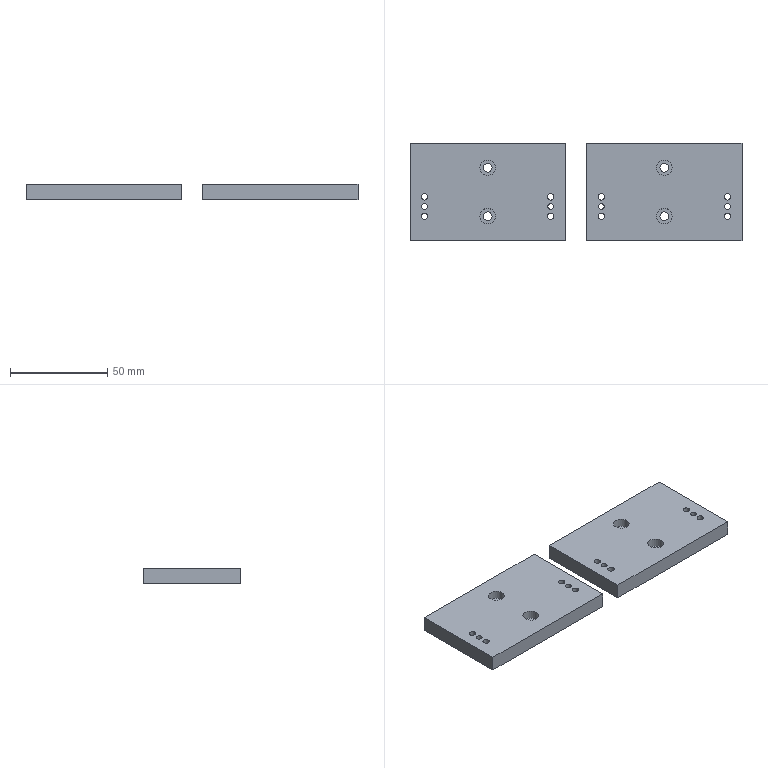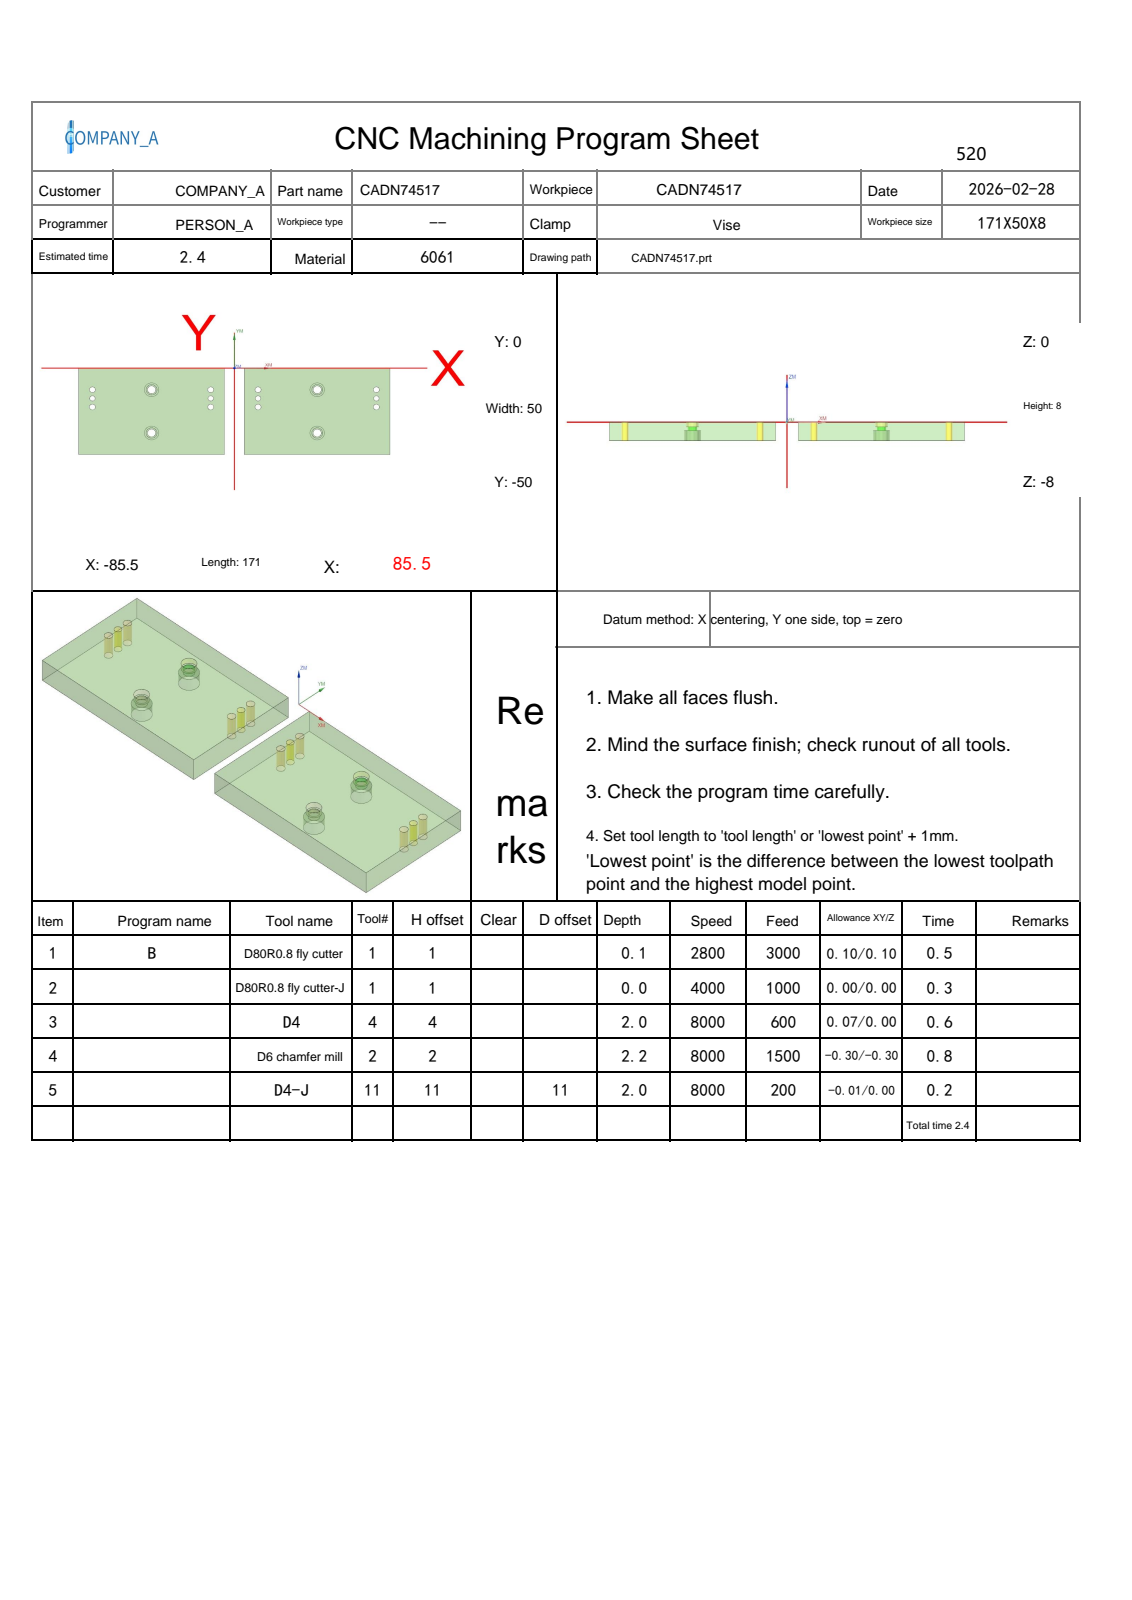NC program | NX | posted by the shop | part box 171 x 50 x 8 mm
Whole program:
%
O0001
(Machine time: 3.31 MIN)
(===Total Tool:4===)
(T1=D80R0.8 fly cutter D=80.  R=0.8  D-  H01 Z=0.    )
(T4=D4      D=4.   R=0.   D-  H04 Z=-2.   )
(T2=D6 chamfer mill   D=6.   R=0.   D-  H02 Z=-2.2  )
(T11=D4-J   D=4.   R=0.   D11 H11 Z=-2.   )
G80 G90 G17 G49 G40
G91 G28 Z0
M01
N1 T01 M06
(D80R0.8 fly cutter  D=80. R=0.8 H=01 ce=0.10 di=0.10)
G00 G90 G54 X137.597 Y-25. M03 S2800
G43 H01 Z50.
M08
Z3.525
G01 Z1.525 F3000.
X125.597
X-125.597
X-137.597
Z3.525
G00 X137.597
Z3.05
G01 Z1.05
X125.597
X-125.597
X-137.597
Z3.05
G00 X137.597
Z2.575
G01 Z.575
X125.597
X-125.597
X-137.597
Z2.575
G00 X137.597
Z2.1
G01 Z.1
X125.597
X-125.597
X-137.597
Z2.1
G00 Z50.
G91 G28 Z0.0
M05
M09
G91 G28 Z0.0
M01
N2 T01 M06
(D80R0.8 fly cutter-J  D=80. R=0.8 H=01 ce=0.00 di=0.00)
G00 G90 G54 X137.499 Y-25. M03 S4000
G43 H01 Z50.
M08
Z2.
G01 Z0.0 F1000.
X125.499
X-125.499
X-137.499
Z2.
G00 Z50.
G91 G28 Z0.0
M05
M09
G91 G28 Z0.0
M01
N3 T04 M06
(D4  D=4. R=0. H=04 ce=0.07 di=0.00)
G00 G90 G54 X45.5 Y-37.5 M03 S8000
G43 H04 Z50.
M08
Z.3
G03 X45.965 Y-37.965 I.465 J0.0 F600.
X46.43 Y-37.5 I0.0 J.465
X46.43 Y-37.5 Z.1 I-.93 J0.0
X46.43 Y-37.5 Z-.1 I-.93 J0.0
X46.43 Y-37.5 Z-.3 I-.93 J0.0
X46.43 Y-37.5 Z-.5 I-.93 J0.0
X46.43 Y-37.5 Z-.7 I-.93 J0.0
X46.43 Y-37.5 Z-.9 I-.93 J0.0
X46.43 Y-37.5 Z-1.1 I-.93 J0.0
X46.43 Y-37.5 Z-1.3 I-.93 J0.0
X46.43 Y-37.5 Z-1.5 I-.93 J0.0
X46.43 Y-37.5 Z-1.7 I-.93 J0.0
X46.43 Y-37.5 Z-1.9 I-.93 J0.0
X44.57 Y-37.5 Z-2. I-.93 J0.0
X45.5 Y-38.43 I.93 J0.0
X46.43 Y-37.5 I0.0 J.93
X45.5 Y-36.57 I-.93 J0.0
X44.57 Y-37.5 I0.0 J-.93
X45.035 Y-37.965 I.465 J0.0
X45.5 Y-37.5 I0.0 J.465
G00 Z50.
X-45.5
Z.3
G03 X-45.035 Y-37.965 I.465 J0.0
X-44.57 Y-37.5 I0.0 J.465
X-44.57 Y-37.5 Z.1 I-.93 J0.0
X-44.57 Y-37.5 Z-.1 I-.93 J0.0
X-44.57 Y-37.5 Z-.3 I-.93 J0.0
X-44.57 Y-37.5 Z-.5 I-.93 J0.0
X-44.57 Y-37.5 Z-.7 I-.93 J0.0
X-44.57 Y-37.5 Z-.9 I-.93 J0.0
X-44.57 Y-37.5 Z-1.1 I-.93 J0.0
X-44.57 Y-37.5 Z-1.3 I-.93 J0.0
X-44.57 Y-37.5 Z-1.5 I-.93 J0.0
X-44.57 Y-37.5 Z-1.7 I-.93 J0.0
X-44.57 Y-37.5 Z-1.9 I-.93 J0.0
X-46.43 Y-37.5 Z-2. I-.93 J0.0
X-45.5 Y-38.43 I.93 J0.0
X-44.57 Y-37.5 I0.0 J.93
X-45.5 Y-36.57 I-.93 J0.0
X-46.43 Y-37.5 I0.0 J-.93
X-45.965 Y-37.965 I.465 J0.0
X-45.5 Y-37.5 I0.0 J.465
G00 Z50.
G00 G90 X45.5 Y-12.5 M03 S8000
Z50.
Z.3
G03 X45.965 Y-12.965 I.465 J0.0 F600.
X46.43 Y-12.5 I0.0 J.465
X46.43 Y-12.5 Z.1 I-.93 J0.0
X46.43 Y-12.5 Z-.1 I-.93 J0.0
X46.43 Y-12.5 Z-.3 I-.93 J0.0
X46.43 Y-12.5 Z-.5 I-.93 J0.0
X46.43 Y-12.5 Z-.7 I-.93 J0.0
X46.43 Y-12.5 Z-.9 I-.93 J0.0
X46.43 Y-12.5 Z-1.1 I-.93 J0.0
X46.43 Y-12.5 Z-1.3 I-.93 J0.0
X46.43 Y-12.5 Z-1.5 I-.93 J0.0
X46.43 Y-12.5 Z-1.7 I-.93 J0.0
X46.43 Y-12.5 Z-1.9 I-.93 J0.0
X44.57 Y-12.5 Z-2. I-.93 J0.0
X45.5 Y-13.43 I.93 J0.0
X46.43 Y-12.5 I0.0 J.93
X45.5 Y-11.57 I-.93 J0.0
X44.57 Y-12.5 I0.0 J-.93
X45.035 Y-12.965 I.465 J0.0
X45.5 Y-12.5 I0.0 J.465
G00 Z50.
X-45.5
Z.3
G03 X-45.035 Y-12.965 I.465 J0.0
X-44.57 Y-12.5 I0.0 J.465
X-44.57 Y-12.5 Z.1 I-.93 J0.0
X-44.57 Y-12.5 Z-.1 I-.93 J0.0
X-44.57 Y-12.5 Z-.3 I-.93 J0.0
X-44.57 Y-12.5 Z-.5 I-.93 J0.0
X-44.57 Y-12.5 Z-.7 I-.93 J0.0
X-44.57 Y-12.5 Z-.9 I-.93 J0.0
X-44.57 Y-12.5 Z-1.1 I-.93 J0.0
X-44.57 Y-12.5 Z-1.3 I-.93 J0.0
X-44.57 Y-12.5 Z-1.5 I-.93 J0.0
X-44.57 Y-12.5 Z-1.7 I-.93 J0.0
X-44.57 Y-12.5 Z-1.9 I-.93 J0.0
X-46.43 Y-12.5 Z-2. I-.93 J0.0
X-45.5 Y-13.43 I.93 J0.0
X-44.57 Y-12.5 I0.0 J.93
X-45.5 Y-11.57 I-.93 J0.0
X-46.43 Y-12.5 I0.0 J-.93
X-45.965 Y-12.965 I.465 J0.0
X-45.5 Y-12.5 I0.0 J.465
G00 Z50.
G91 G28 Z0.0
M05
M09
G91 G28 Z0.0
M01
N4 T02 M06
(D6 chamfer mill  D=6. R=0. H=02 ce=0.00 di=0.00)
G00 G90 G54 X78. Y-17.5 M03 S8000
G43 H02 Z50.
M08
G98 G81 X78. Y-17.5 Z-1.8 R3. F1000.
X13.
X-13.
X-78.
G80
G00 Z50.
G00 G90 X78. Y-12.5 M03 S8000
Z50.
G98 G81 X78. Y-12.5 Z-2.2 R3. F1000.
Y-22.5
X13.
Y-12.5
X-13.
Y-22.5
X-78.
Y-12.5
G80
G00 Z50.
G00 G90 X-45.434 Y-37.793 M03 S8000
Z50.
Z-1.5
G01 Z-2. F600.
X-45.306 Y-37.808
X-45.125 Y-37.819
G03 X-44.2 Y-37.5 I0.0 J1.5
X-45.5 Y-36.2 I-1.3 J0.0
X-46.8 Y-37.5 I0.0 J-1.3
X-45.5 Y-38.8 I1.3 J0.0
X-44.2 Y-37.5 I0.0 J1.3
X-45.125 Y-37.181 I-.925 J-1.181
G01 X-45.306 Y-37.192
X-45.434 Y-37.207
Z-1.5
G00 Z50.
Y-12.793
Z-1.5
G01 Z-2.
X-45.306 Y-12.808
X-45.125 Y-12.819
G03 X-44.2 Y-12.5 I0.0 J1.5
X-45.5 Y-11.2 I-1.3 J0.0
X-46.8 Y-12.5 I0.0 J-1.3
X-45.5 Y-13.8 I1.3 J0.0
X-44.2 Y-12.5 I0.0 J1.3
X-45.125 Y-12.181 I-.925 J-1.181
G01 X-45.306 Y-12.192
X-45.434 Y-12.207
Z-1.5
G00 Z50.
X45.566 Y-12.793
Z-1.5
G01 Z-2.
X45.694 Y-12.808
X45.875 Y-12.819
G03 X46.8 Y-12.5 I0.0 J1.5
X45.5 Y-11.2 I-1.3 J0.0
X44.2 Y-12.5 I0.0 J-1.3
X45.5 Y-13.8 I1.3 J0.0
X46.8 Y-12.5 I0.0 J1.3
X45.875 Y-12.181 I-.925 J-1.181
G01 X45.694 Y-12.192
X45.566 Y-12.207
Z-1.5
G00 Z50.
Y-37.793
Z-1.5
G01 Z-2.
X45.694 Y-37.808
X45.875 Y-37.819
G03 X46.8 Y-37.5 I0.0 J1.5
X45.5 Y-36.2 I-1.3 J0.0
X44.2 Y-37.5 I0.0 J-1.3
X45.5 Y-38.8 I1.3 J0.0
X46.8 Y-37.5 I0.0 J1.3
X45.875 Y-37.181 I-.925 J-1.181
G01 X45.694 Y-37.192
X45.566 Y-37.207
Z-1.5
G00 Z50.
G00 G90 X45.886 Y-51.227 M03 S6500
Z50.
Z.172
G01 Z-1.2 F1500.
G03 X45.6 Y-51.027 I-1.286 J-1.532
G01 X45.554 Y-50.997
X45.5 Y-51.
X5.5
G02 X4.5 Y-50. I0.0 J1.
G01 Y0.0
G02 X5.5 Y1. I1. J0.0
G01 X85.5
G02 X86.5 Y0.0 I0.0 J-1.
G01 Y-50.
G02 X85.5 Y-51. I-1. J0.0
G01 X45.5
X45.446 Y-50.997
X45.4 Y-51.027
G03 X45.114 Y-51.227 I1. J-1.732
G01 Z.172
G00 Z10.
X12.506 Y-12.081
Z.405
G01 Z-1.2
G03 X12.359 Y-12.397 I1.732 J-1.
G01 X12.338 Y-12.447
X12.35 Y-12.5
G03 X13. Y-13.15 I.65 J0.0
X13.65 Y-12.5 I0.0 J.65
X13. Y-11.85 I-.65 J0.0
X12.35 Y-12.5 I0.0 J-.65
G01 X12.338 Y-12.553
X12.359 Y-12.603
G03 X12.506 Y-12.919 I1.879 J.684
G01 Z.405
G00 Z2.55
X12.656 Y-17.081
Z.447
G01 Z-1.2
G03 X12.509 Y-17.397 I1.732 J-1.
G01 X12.488 Y-17.447
X12.5 Y-17.5
G03 X13. Y-18. I.5 J0.0
X13.5 Y-17.5 I0.0 J.5
X13. Y-17. I-.5 J0.0
X12.5 Y-17.5 I0.0 J-.5
G01 X12.488 Y-17.553
X12.509 Y-17.603
G03 X12.656 Y-17.919 I1.879 J.684
G01 Z.447
G00 Z2.55
X12.506 Y-22.081
Z.405
G01 Z-1.2
G03 X12.359 Y-22.397 I1.732 J-1.
G01 X12.338 Y-22.447
X12.35 Y-22.5
G03 X13. Y-23.15 I.65 J0.0
X13.65 Y-22.5 I0.0 J.65
X13. Y-21.85 I-.65 J0.0
X12.35 Y-22.5 I0.0 J-.65
G01 X12.338 Y-22.553
X12.359 Y-22.603
G03 X12.506 Y-22.919 I1.879 J.684
G01 Z.405
G00 Z10.
X47.308 Y-37.904
Z.257
G01 Z-1.2
G03 X47.482 Y-37.602 I-1.638 J1.147
G01 X47.508 Y-37.554
X47.5 Y-37.5
G03 X45.5 Y-35.5 I-2. J0.0
X43.5 Y-37.5 I0.0 J-2.
X45.5 Y-39.5 I2. J0.0
X47.47 Y-37.847 I0.0 J2.
G01 X47.5 Y-37.5
X47.508 Y-37.446
X47.482 Y-37.398
G03 X47.308 Y-37.096 I-1.813 J-.845
G01 Z.257
G00 Z10.
Y-12.904
Z.257
G01 Z-1.2
G03 X47.482 Y-12.602 I-1.638 J1.147
G01 X47.508 Y-12.554
X47.5 Y-12.5
G03 X45.5 Y-10.5 I-2. J0.0
X43.5 Y-12.5 I0.0 J-2.
X45.5 Y-14.5 I2. J0.0
X47.47 Y-12.847 I0.0 J2.
G01 X47.5 Y-12.5
X47.508 Y-12.446
X47.482 Y-12.398
G03 X47.308 Y-12.096 I-1.813 J-.845
G01 Z.257
G00 Z10.
X77.506 Y-12.081
Z.405
G01 Z-1.2
G03 X77.359 Y-12.397 I1.732 J-1.
G01 X77.338 Y-12.447
X77.35 Y-12.5
G03 X78. Y-13.15 I.65 J0.0
X78.65 Y-12.5 I0.0 J.65
X78. Y-11.85 I-.65 J0.0
X77.35 Y-12.5 I0.0 J-.65
G01 X77.338 Y-12.553
X77.359 Y-12.603
G03 X77.506 Y-12.919 I1.879 J.684
G01 Z.405
G00 Z2.55
X77.656 Y-17.081
Z.447
G01 Z-1.2
G03 X77.509 Y-17.397 I1.732 J-1.
G01 X77.488 Y-17.447
X77.5 Y-17.5
G03 X78. Y-18. I.5 J0.0
X78.5 Y-17.5 I0.0 J.5
X78. Y-17. I-.5 J0.0
X77.5 Y-17.5 I0.0 J-.5
G01 X77.488 Y-17.553
X77.509 Y-17.603
G03 X77.656 Y-17.919 I1.879 J.684
G01 Z.447
G00 Z2.55
X77.506 Y-22.081
Z.405
G01 Z-1.2
G03 X77.359 Y-22.397 I1.732 J-1.
G01 X77.338 Y-22.447
X77.35 Y-22.5
G03 X78. Y-23.15 I.65 J0.0
X78.65 Y-22.5 I0.0 J.65
X78. Y-21.85 I-.65 J0.0
X77.35 Y-22.5 I0.0 J-.65
G01 X77.338 Y-22.553
X77.359 Y-22.603
G03 X77.506 Y-22.919 I1.879 J.684
G01 Z.405
G00 Z10.
X-45.114 Y-51.227
Z.172
G01 Z-1.2
G03 X-45.4 Y-51.027 I-1.286 J-1.532
G01 X-45.446 Y-50.997
X-45.5 Y-51.
X-85.5
G02 X-86.5 Y-50. I0.0 J1.
G01 Y0.0
G02 X-85.5 Y1. I1. J0.0
G01 X-5.5
G02 X-4.5 Y0.0 I0.0 J-1.
G01 Y-50.
G02 X-5.5 Y-51. I-1. J0.0
G01 X-45.5
X-45.554 Y-50.997
X-45.6 Y-51.027
G03 X-45.886 Y-51.227 I1. J-1.732
G01 Z.172
G00 Z10.
X-78.494 Y-12.081
Z.405
G01 Z-1.2
G03 X-78.641 Y-12.397 I1.732 J-1.
G01 X-78.662 Y-12.447
X-78.65 Y-12.5
G03 X-78. Y-13.15 I.65 J0.0
X-77.35 Y-12.5 I0.0 J.65
X-78. Y-11.85 I-.65 J0.0
X-78.65 Y-12.5 I0.0 J-.65
G01 X-78.662 Y-12.553
X-78.641 Y-12.603
G03 X-78.494 Y-12.919 I1.879 J.684
G01 Z.405
G00 Z2.55
X-78.344 Y-17.081
Z.447
G01 Z-1.2
G03 X-78.491 Y-17.397 I1.732 J-1.
G01 X-78.512 Y-17.447
X-78.5 Y-17.5
G03 X-78. Y-18. I.5 J0.0
X-77.5 Y-17.5 I0.0 J.5
X-78. Y-17. I-.5 J0.0
X-78.5 Y-17.5 I0.0 J-.5
G01 X-78.512 Y-17.553
X-78.491 Y-17.603
G03 X-78.344 Y-17.919 I1.879 J.684
G01 Z.447
G00 Z2.55
X-78.494 Y-22.081
Z.405
G01 Z-1.2
G03 X-78.641 Y-22.397 I1.732 J-1.
G01 X-78.662 Y-22.447
X-78.65 Y-22.5
G03 X-78. Y-23.15 I.65 J0.0
X-77.35 Y-22.5 I0.0 J.65
X-78. Y-21.85 I-.65 J0.0
X-78.65 Y-22.5 I0.0 J-.65
G01 X-78.662 Y-22.553
X-78.641 Y-22.603
G03 X-78.494 Y-22.919 I1.879 J.684
G01 Z.405
G00 Z10.
X-43.692 Y-37.904
Z.257
G01 Z-1.2
G03 X-43.518 Y-37.602 I-1.638 J1.147
G01 X-43.492 Y-37.554
X-43.5 Y-37.5
G03 X-45.5 Y-35.5 I-2. J0.0
X-47.5 Y-37.5 I0.0 J-2.
X-45.5 Y-39.5 I2. J0.0
X-43.53 Y-37.847 I0.0 J2.
G01 X-43.5 Y-37.5
X-43.492 Y-37.446
X-43.518 Y-37.398
G03 X-43.692 Y-37.096 I-1.813 J-.845
G01 Z.257
G00 Z10.
Y-12.904
Z.257
G01 Z-1.2
G03 X-43.518 Y-12.602 I-1.638 J1.147
G01 X-43.492 Y-12.554
X-43.5 Y-12.5
G03 X-45.5 Y-10.5 I-2. J0.0
X-47.5 Y-12.5 I0.0 J-2.
X-45.5 Y-14.5 I2. J0.0
X-43.53 Y-12.847 I0.0 J2.
G01 X-43.5 Y-12.5
X-43.492 Y-12.446
X-43.518 Y-12.398
G03 X-43.692 Y-12.096 I-1.813 J-.845
G01 Z.257
G00 Z10.
X-13.494 Y-12.081
Z.405
G01 Z-1.2
G03 X-13.641 Y-12.397 I1.732 J-1.
G01 X-13.662 Y-12.447
X-13.65 Y-12.5
G03 X-13. Y-13.15 I.65 J0.0
X-12.35 Y-12.5 I0.0 J.65
X-13. Y-11.85 I-.65 J0.0
X-13.65 Y-12.5 I0.0 J-.65
G01 X-13.662 Y-12.553
X-13.641 Y-12.603
G03 X-13.494 Y-12.919 I1.879 J.684
G01 Z.405
G00 Z2.55
X-13.344 Y-17.081
Z.447
G01 Z-1.2
G03 X-13.491 Y-17.397 I1.732 J-1.
G01 X-13.512 Y-17.447
X-13.5 Y-17.5
G03 X-13. Y-18. I.5 J0.0
X-12.5 Y-17.5 I0.0 J.5
X-13. Y-17. I-.5 J0.0
X-13.5 Y-17.5 I0.0 J-.5
G01 X-13.512 Y-17.553
X-13.491 Y-17.603
G03 X-13.344 Y-17.919 I1.879 J.684
G01 Z.447
G00 Z2.55
X-13.494 Y-22.081
Z.405
G01 Z-1.2
G03 X-13.641 Y-22.397 I1.732 J-1.
G01 X-13.662 Y-22.447
X-13.65 Y-22.5
G03 X-13. Y-23.15 I.65 J0.0
X-12.35 Y-22.5 I0.0 J.65
X-13. Y-21.85 I-.65 J0.0
X-13.65 Y-22.5 I0.0 J-.65
G01 X-13.662 Y-22.553
X-13.641 Y-22.603
G03 X-13.494 Y-22.919 I1.879 J.684
G01 Z.405
G00 Z50.
G91 G28 Z0.0
M05
M09
G91 G28 Z0.0
M01
N5 T11 M06
(D4-J  D=4. R=0. H=11 ce=-0.01 di=0.00)
G00 G90 G54 X45.5 Y-37.5 M03 S8000
G43 H11 Z50.
M08
Z-2.
G41 D11
G01 X46.041 Y-37.823 F200.
X46.164 Y-37.846
G03 X46.51 Y-37.5 I0.0 J.346
X45.5 Y-36.49 I-1.01 J0.0
X44.49 Y-37.5 I0.0 J-1.01
X45.5 Y-38.51 I1.01 J0.0
X46.51 Y-37.5 I0.0 J1.01
X46.389 Y-37.02 I-1.01 J0.0
X46.084 Y-36.839 I-.304 J-.164
X45.822 Y-36.959 I0.0 J-.346
G01 G40 X45.5 Y-37.5
G00 Z50.
X-45.5
Z-2.
G41 D11
G01 X-44.959 Y-37.823
X-44.836 Y-37.846
G03 X-44.49 Y-37.5 I0.0 J.346
X-45.5 Y-36.49 I-1.01 J0.0
X-46.51 Y-37.5 I0.0 J-1.01
X-45.5 Y-38.51 I1.01 J0.0
X-44.49 Y-37.5 I0.0 J1.01
X-44.611 Y-37.02 I-1.01 J0.0
X-44.916 Y-36.839 I-.304 J-.164
X-45.178 Y-36.959 I0.0 J-.346
G01 G40 X-45.5 Y-37.5
G00 Z50.
G00 G90 X45.5 Y-12.5 M03 S8000
Z50.
Z-2.
G41 D11
G01 X46.041 Y-12.823 F200.
X46.164 Y-12.846
G03 X46.51 Y-12.5 I0.0 J.346
X45.5 Y-11.49 I-1.01 J0.0
X44.49 Y-12.5 I0.0 J-1.01
X45.5 Y-13.51 I1.01 J0.0
X46.51 Y-12.5 I0.0 J1.01
X46.389 Y-12.02 I-1.01 J0.0
X46.084 Y-11.839 I-.304 J-.164
X45.822 Y-11.959 I0.0 J-.346
G01 G40 X45.5 Y-12.5
G00 Z50.
X-45.5
Z-2.
G41 D11
G01 X-44.959 Y-12.823
X-44.836 Y-12.846
G03 X-44.49 Y-12.5 I0.0 J.346
X-45.5 Y-11.49 I-1.01 J0.0
X-46.51 Y-12.5 I0.0 J-1.01
X-45.5 Y-13.51 I1.01 J0.0
X-44.49 Y-12.5 I0.0 J1.01
X-44.611 Y-12.02 I-1.01 J0.0
X-44.916 Y-11.839 I-.304 J-.164
X-45.178 Y-11.959 I0.0 J-.346
G01 G40 X-45.5 Y-12.5
G00 Z50.
M05
M09
G91 G28 Z0.0
G91 G28 Y0.0
M30
%